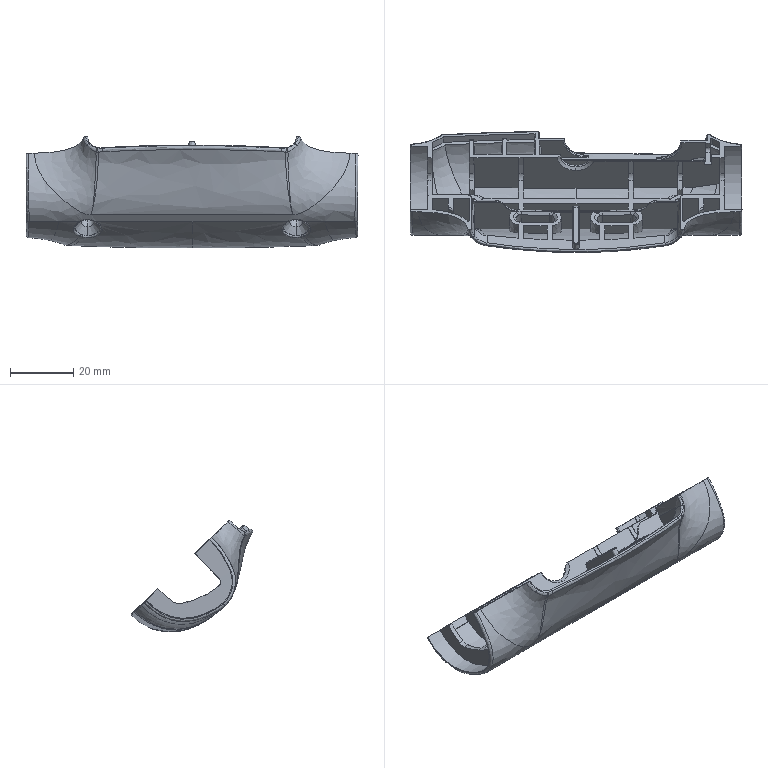Part | SolidWorks | features BaseBody 1 | 1 solid | 427 faces | box 105 x 38.346 x 35.414 mm | volume 18588 mm3 | spline 196 | plane 127 | cylinder 63 | cone 41 | commonest cylinder face diameters 0.6 x7 50.022 x7 17.297 x5 3.3 x4 3.4 x4 4.2 x4